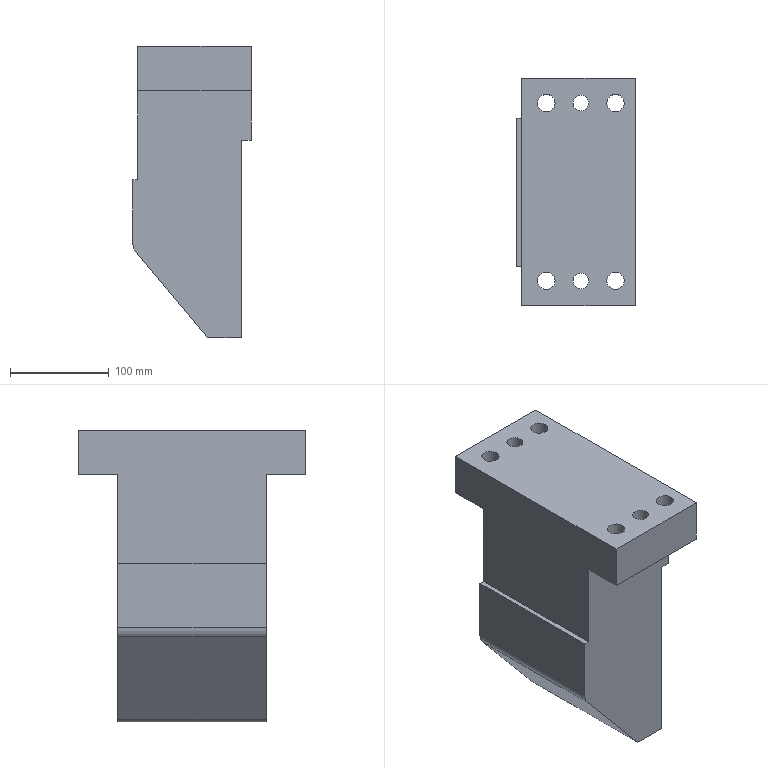Part | NX | features solid 2 | 1 solid | 31 faces | box 120 x 230 x 295 mm | volume 4727759 mm3 | plane 19 | cylinder 12 | commonest cylinder face diameters 17.5 x4 26 x4 16 x2 10 x1 30 x1
STEP:
#1=CARTESIAN_POINT('',(785.,300.,35.));
#2=VERTEX_POINT('',#1);
#3=CARTESIAN_POINT('',(785.,70.,35.));
#4=VERTEX_POINT('',#3);
#5=CARTESIAN_POINT('',(785.,82.5,35.));
#6=DIRECTION('',(0.,1.,0.));
#7=VECTOR('',#6,1000.);
#8=LINE('',#5,#7);
#9=EDGE_CURVE('',#2,#4,#8,.F.);
#10=ORIENTED_EDGE('',*,*,#9,.F.);
#11=CARTESIAN_POINT('',(785.,300.,-10.));
#12=VERTEX_POINT('',#11);
#13=CARTESIAN_POINT('',(785.,300.,-158.));
#14=DIRECTION('',(0.,0.,-1.));
#15=VECTOR('',#14,1000.);
#16=LINE('',#13,#15);
#17=EDGE_CURVE('',#2,#12,#16,.T.);
#18=ORIENTED_EDGE('',*,*,#17,.T.);
#19=CARTESIAN_POINT('',(785.,260.,-10.));
#20=VERTEX_POINT('',#19);
#21=CARTESIAN_POINT('',(785.,383.5,-10.));
#22=DIRECTION('',(0.,1.,0.));
#23=VECTOR('',#22,1000.);
#24=LINE('',#21,#23);
#25=EDGE_CURVE('',#12,#20,#24,.F.);
#26=ORIENTED_EDGE('',*,*,#25,.T.);
#27=CARTESIAN_POINT('',(785.,260.,-100.));
#28=VERTEX_POINT('',#27);
#29=CARTESIAN_POINT('',(785.,260.,-334.604));
#30=DIRECTION('',(0.,0.,-1.));
#31=VECTOR('',#30,1000.);
#32=LINE('',#29,#31);
#33=EDGE_CURVE('',#20,#28,#32,.T.);
#34=ORIENTED_EDGE('',*,*,#33,.T.);
#35=CARTESIAN_POINT('',(785.,110.,-100.));
#36=VERTEX_POINT('',#35);
#37=CARTESIAN_POINT('',(785.,340.,-100.));
#38=DIRECTION('',(0.,-1.,0.));
#39=VECTOR('',#38,1000.);
#40=LINE('',#37,#39);
#41=EDGE_CURVE('',#28,#36,#40,.T.);
#42=ORIENTED_EDGE('',*,*,#41,.T.);
#43=CARTESIAN_POINT('',(785.,110.,-10.));
#44=VERTEX_POINT('',#43);
#45=CARTESIAN_POINT('',(785.,110.,-334.604));
#46=DIRECTION('',(0.,0.,-1.));
#47=VECTOR('',#46,1000.);
#48=LINE('',#45,#47);
#49=EDGE_CURVE('',#44,#36,#48,.T.);
#50=ORIENTED_EDGE('',*,*,#49,.F.);
#51=CARTESIAN_POINT('',(785.,70.,-10.));
#52=VERTEX_POINT('',#51);
#53=CARTESIAN_POINT('',(785.,21.5,-10.));
#54=DIRECTION('',(0.,-1.,0.));
#55=VECTOR('',#54,1000.);
#56=LINE('',#53,#55);
#57=EDGE_CURVE('',#52,#44,#56,.F.);
#58=ORIENTED_EDGE('',*,*,#57,.F.);
#59=CARTESIAN_POINT('',(785.,70.,-158.));
#60=DIRECTION('',(0.,0.,-1.));
#61=VECTOR('',#60,1000.);
#62=LINE('',#59,#61);
#63=EDGE_CURVE('',#4,#52,#62,.T.);
#64=ORIENTED_EDGE('',*,*,#63,.F.);
#65=EDGE_LOOP('',(#10,#18,#26,#34,#42,#50,#58,#64));
#66=FACE_BOUND('',#65,.T.);
#67=CARTESIAN_POINT('',(785.,82.5,-158.));
#68=DIRECTION('',(-1.,0.,0.));
#69=DIRECTION('',(0.,0.,-1.));
#70=AXIS2_PLACEMENT_3D('',#67,#68,#69);
#71=PLANE('',#70);
#72=ADVANCED_FACE('',(#66),#71,.T.);
#73=CARTESIAN_POINT('',(900.,70.,35.));
#74=VERTEX_POINT('',#73);
#75=CARTESIAN_POINT('',(900.,300.,35.));
#76=VERTEX_POINT('',#75);
#77=CARTESIAN_POINT('',(900.,82.5,35.));
#78=DIRECTION('',(0.,-1.,0.));
#79=VECTOR('',#78,1000.);
#80=LINE('',#77,#79);
#81=EDGE_CURVE('',#74,#76,#80,.F.);
#82=ORIENTED_EDGE('',*,*,#81,.T.);
#83=CARTESIAN_POINT('',(785.,300.,35.));
#84=DIRECTION('',(-1.,0.,0.));
#85=VECTOR('',#84,1000.);
#86=LINE('',#83,#85);
#87=EDGE_CURVE('',#2,#76,#86,.F.);
#88=ORIENTED_EDGE('',*,*,#87,.F.);
#89=ORIENTED_EDGE('',*,*,#9,.T.);
#90=CARTESIAN_POINT('',(785.,70.,35.));
#91=DIRECTION('',(-1.,0.,0.));
#92=VECTOR('',#91,1000.);
#93=LINE('',#90,#92);
#94=EDGE_CURVE('',#4,#74,#93,.F.);
#95=ORIENTED_EDGE('',*,*,#94,.T.);
#96=EDGE_LOOP('',(#82,#88,#89,#95));
#97=FACE_BOUND('',#96,.T.);
#98=CARTESIAN_POINT('',(801.25,275.,35.));
#99=VERTEX_POINT('',#98);
#100=CARTESIAN_POINT('',(810.,275.,35.));
#101=DIRECTION('',(0.,0.,1.));
#102=DIRECTION('',(-1.,0.,0.));
#103=AXIS2_PLACEMENT_3D('',#100,#101,#102);
#104=CIRCLE('',#103,8.75);
#105=EDGE_CURVE('',#99,#99,#104,.F.);
#106=ORIENTED_EDGE('',*,*,#105,.T.);
#107=EDGE_LOOP('',(#106));
#108=FACE_BOUND('',#107,.T.);
#109=CARTESIAN_POINT('',(871.25,275.,35.));
#110=VERTEX_POINT('',#109);
#111=CARTESIAN_POINT('',(880.,275.,35.));
#112=DIRECTION('',(0.,0.,1.));
#113=DIRECTION('',(-1.,0.,0.));
#114=AXIS2_PLACEMENT_3D('',#111,#112,#113);
#115=CIRCLE('',#114,8.75);
#116=EDGE_CURVE('',#110,#110,#115,.F.);
#117=ORIENTED_EDGE('',*,*,#116,.T.);
#118=EDGE_LOOP('',(#117));
#119=FACE_BOUND('',#118,.T.);
#120=CARTESIAN_POINT('',(837.,275.,35.));
#121=VERTEX_POINT('',#120);
#122=CARTESIAN_POINT('',(845.,275.,35.));
#123=DIRECTION('',(0.,0.,1.));
#124=DIRECTION('',(-1.,0.,0.));
#125=AXIS2_PLACEMENT_3D('',#122,#123,#124);
#126=CIRCLE('',#125,8.);
#127=EDGE_CURVE('',#121,#121,#126,.F.);
#128=ORIENTED_EDGE('',*,*,#127,.T.);
#129=EDGE_LOOP('',(#128));
#130=FACE_BOUND('',#129,.T.);
#131=CARTESIAN_POINT('',(837.,95.,35.));
#132=VERTEX_POINT('',#131);
#133=CARTESIAN_POINT('',(845.,95.,35.));
#134=DIRECTION('',(0.,0.,-1.));
#135=DIRECTION('',(-1.,0.,0.));
#136=AXIS2_PLACEMENT_3D('',#133,#134,#135);
#137=CIRCLE('',#136,8.);
#138=EDGE_CURVE('',#132,#132,#137,.F.);
#139=ORIENTED_EDGE('',*,*,#138,.F.);
#140=EDGE_LOOP('',(#139));
#141=FACE_BOUND('',#140,.T.);
#142=CARTESIAN_POINT('',(871.25,95.,35.));
#143=VERTEX_POINT('',#142);
#144=CARTESIAN_POINT('',(880.,95.,35.));
#145=DIRECTION('',(0.,0.,-1.));
#146=DIRECTION('',(-1.,0.,0.));
#147=AXIS2_PLACEMENT_3D('',#144,#145,#146);
#148=CIRCLE('',#147,8.75);
#149=EDGE_CURVE('',#143,#143,#148,.F.);
#150=ORIENTED_EDGE('',*,*,#149,.F.);
#151=EDGE_LOOP('',(#150));
#152=FACE_BOUND('',#151,.T.);
#153=CARTESIAN_POINT('',(801.25,95.,35.));
#154=VERTEX_POINT('',#153);
#155=CARTESIAN_POINT('',(810.,95.,35.));
#156=DIRECTION('',(0.,0.,-1.));
#157=DIRECTION('',(-1.,0.,0.));
#158=AXIS2_PLACEMENT_3D('',#155,#156,#157);
#159=CIRCLE('',#158,8.75);
#160=EDGE_CURVE('',#154,#154,#159,.F.);
#161=ORIENTED_EDGE('',*,*,#160,.F.);
#162=EDGE_LOOP('',(#161));
#163=FACE_BOUND('',#162,.T.);
#164=CARTESIAN_POINT('',(800.,82.5,35.));
#165=DIRECTION('',(0.,0.,1.));
#166=DIRECTION('',(-1.,0.,0.));
#167=AXIS2_PLACEMENT_3D('',#164,#165,#166);
#168=PLANE('',#167);
#169=ADVANCED_FACE('',(#97,#108,#119,#130,#141,#152,#163),#168,.T.);
#170=CARTESIAN_POINT('',(900.,260.,-60.));
#171=VERTEX_POINT('',#170);
#172=CARTESIAN_POINT('',(900.,260.,-10.));
#173=VERTEX_POINT('',#172);
#174=CARTESIAN_POINT('',(900.,260.,37.));
#175=DIRECTION('',(0.,0.,1.));
#176=VECTOR('',#175,1000.);
#177=LINE('',#174,#176);
#178=EDGE_CURVE('',#171,#173,#177,.T.);
#179=ORIENTED_EDGE('',*,*,#178,.T.);
#180=CARTESIAN_POINT('',(900.,300.,-10.));
#181=VERTEX_POINT('',#180);
#182=CARTESIAN_POINT('',(900.,383.5,-10.));
#183=DIRECTION('',(0.,-1.,0.));
#184=VECTOR('',#183,1000.);
#185=LINE('',#182,#184);
#186=EDGE_CURVE('',#181,#173,#185,.T.);
#187=ORIENTED_EDGE('',*,*,#186,.F.);
#188=CARTESIAN_POINT('',(900.,300.,37.));
#189=DIRECTION('',(0.,0.,-1.));
#190=VECTOR('',#189,1000.);
#191=LINE('',#188,#190);
#192=EDGE_CURVE('',#76,#181,#191,.T.);
#193=ORIENTED_EDGE('',*,*,#192,.F.);
#194=ORIENTED_EDGE('',*,*,#81,.F.);
#195=CARTESIAN_POINT('',(900.,70.,-10.));
#196=VERTEX_POINT('',#195);
#197=CARTESIAN_POINT('',(900.,70.,37.));
#198=DIRECTION('',(0.,0.,-1.));
#199=VECTOR('',#198,1000.);
#200=LINE('',#197,#199);
#201=EDGE_CURVE('',#74,#196,#200,.T.);
#202=ORIENTED_EDGE('',*,*,#201,.T.);
#203=CARTESIAN_POINT('',(900.,110.,-10.));
#204=VERTEX_POINT('',#203);
#205=CARTESIAN_POINT('',(900.,172.5,-10.));
#206=DIRECTION('',(0.,1.,0.));
#207=VECTOR('',#206,1000.);
#208=LINE('',#205,#207);
#209=EDGE_CURVE('',#196,#204,#208,.T.);
#210=ORIENTED_EDGE('',*,*,#209,.T.);
#211=CARTESIAN_POINT('',(900.,110.,-60.));
#212=VERTEX_POINT('',#211);
#213=CARTESIAN_POINT('',(900.,110.,-334.604));
#214=DIRECTION('',(0.,0.,-1.));
#215=VECTOR('',#214,1000.);
#216=LINE('',#213,#215);
#217=EDGE_CURVE('',#204,#212,#216,.T.);
#218=ORIENTED_EDGE('',*,*,#217,.T.);
#219=CARTESIAN_POINT('',(900.,282.5,-60.));
#220=DIRECTION('',(0.,1.,0.));
#221=VECTOR('',#220,1000.);
#222=LINE('',#219,#221);
#223=EDGE_CURVE('',#212,#171,#222,.T.);
#224=ORIENTED_EDGE('',*,*,#223,.T.);
#225=EDGE_LOOP('',(#179,#187,#193,#194,#202,#210,#218,#224));
#226=FACE_BOUND('',#225,.T.);
#227=CARTESIAN_POINT('',(900.,172.5,37.));
#228=DIRECTION('',(-1.,0.,0.));
#229=DIRECTION('',(0.,0.,-1.));
#230=AXIS2_PLACEMENT_3D('',#227,#228,#229);
#231=PLANE('',#230);
#232=ADVANCED_FACE('',(#226),#231,.F.);
#233=CARTESIAN_POINT('',(695.,110.,-10.));
#234=DIRECTION('',(1.,0.,0.));
#235=VECTOR('',#234,1000.);
#236=LINE('',#233,#235);
#237=EDGE_CURVE('',#44,#204,#236,.T.);
#238=ORIENTED_EDGE('',*,*,#237,.F.);
#239=ORIENTED_EDGE('',*,*,#49,.T.);
#240=CARTESIAN_POINT('',(780.,110.,-100.));
#241=VERTEX_POINT('',#240);
#242=CARTESIAN_POINT('',(840.,110.,-100.));
#243=DIRECTION('',(1.,0.,0.));
#244=VECTOR('',#243,1000.);
#245=LINE('',#242,#244);
#246=EDGE_CURVE('',#241,#36,#245,.T.);
#247=ORIENTED_EDGE('',*,*,#246,.F.);
#248=CARTESIAN_POINT('',(780.,110.,-164.54));
#249=VERTEX_POINT('',#248);
#250=CARTESIAN_POINT('',(780.,110.,-334.604));
#251=DIRECTION('',(0.,0.,-1.));
#252=VECTOR('',#251,1000.);
#253=LINE('',#250,#252);
#254=EDGE_CURVE('',#241,#249,#253,.T.);
#255=ORIENTED_EDGE('',*,*,#254,.T.);
#256=CARTESIAN_POINT('',(783.509,110.,-174.182));
#257=VERTEX_POINT('',#256);
#258=CARTESIAN_POINT('',(795.,110.,-164.54));
#259=DIRECTION('',(0.,-1.,0.));
#260=DIRECTION('',(0.,0.,1.));
#261=AXIS2_PLACEMENT_3D('',#258,#259,#260);
#262=CIRCLE('',#261,15.);
#263=EDGE_CURVE('',#249,#257,#262,.T.);
#264=ORIENTED_EDGE('',*,*,#263,.T.);
#265=CARTESIAN_POINT('',(854.02,110.,-258.214));
#266=VERTEX_POINT('',#265);
#267=CARTESIAN_POINT('',(780.,110.,-170.));
#268=DIRECTION('',(0.6428,0.,-0.766));
#269=VECTOR('',#268,1000.);
#270=LINE('',#267,#269);
#271=EDGE_CURVE('',#257,#266,#270,.T.);
#272=ORIENTED_EDGE('',*,*,#271,.T.);
#273=CARTESIAN_POINT('',(857.851,110.,-260.));
#274=VERTEX_POINT('',#273);
#275=CARTESIAN_POINT('',(857.851,110.,-255.));
#276=DIRECTION('',(0.,-1.,0.));
#277=DIRECTION('',(0.,0.,1.));
#278=AXIS2_PLACEMENT_3D('',#275,#276,#277);
#279=CIRCLE('',#278,5.);
#280=EDGE_CURVE('',#266,#274,#279,.T.);
#281=ORIENTED_EDGE('',*,*,#280,.T.);
#282=CARTESIAN_POINT('',(890.,110.,-260.));
#283=VERTEX_POINT('',#282);
#284=CARTESIAN_POINT('',(764.279,110.,-260.));
#285=DIRECTION('',(1.,0.,0.));
#286=VECTOR('',#285,1000.);
#287=LINE('',#284,#286);
#288=EDGE_CURVE('',#274,#283,#287,.T.);
#289=ORIENTED_EDGE('',*,*,#288,.T.);
#290=CARTESIAN_POINT('',(890.,110.,-60.));
#291=VERTEX_POINT('',#290);
#292=CARTESIAN_POINT('',(890.,110.,-334.604));
#293=DIRECTION('',(0.,0.,1.));
#294=VECTOR('',#293,1000.);
#295=LINE('',#292,#294);
#296=EDGE_CURVE('',#283,#291,#295,.T.);
#297=ORIENTED_EDGE('',*,*,#296,.T.);
#298=CARTESIAN_POINT('',(764.279,110.,-60.));
#299=DIRECTION('',(1.,0.,0.));
#300=VECTOR('',#299,1000.);
#301=LINE('',#298,#300);
#302=EDGE_CURVE('',#291,#212,#301,.T.);
#303=ORIENTED_EDGE('',*,*,#302,.T.);
#304=ORIENTED_EDGE('',*,*,#217,.F.);
#305=EDGE_LOOP('',(#238,#239,#247,#255,#264,#272,#281,#289,#297,#303,#304));
#306=FACE_BOUND('',#305,.T.);
#307=CARTESIAN_POINT('',(764.279,110.,-334.604));
#308=DIRECTION('',(0.,-1.,0.));
#309=DIRECTION('',(0.,0.,1.));
#310=AXIS2_PLACEMENT_3D('',#307,#308,#309);
#311=PLANE('',#310);
#312=ADVANCED_FACE('',(#306),#311,.T.);
#313=ORIENTED_EDGE('',*,*,#33,.F.);
#314=CARTESIAN_POINT('',(695.,260.,-10.));
#315=DIRECTION('',(1.,0.,0.));
#316=VECTOR('',#315,1000.);
#317=LINE('',#314,#316);
#318=EDGE_CURVE('',#20,#173,#317,.T.);
#319=ORIENTED_EDGE('',*,*,#318,.T.);
#320=ORIENTED_EDGE('',*,*,#178,.F.);
#321=CARTESIAN_POINT('',(890.,260.,-60.));
#322=VERTEX_POINT('',#321);
#323=CARTESIAN_POINT('',(935.,260.,-60.));
#324=DIRECTION('',(-1.,0.,0.));
#325=VECTOR('',#324,1000.);
#326=LINE('',#323,#325);
#327=EDGE_CURVE('',#171,#322,#326,.T.);
#328=ORIENTED_EDGE('',*,*,#327,.T.);
#329=CARTESIAN_POINT('',(890.,260.,-260.));
#330=VERTEX_POINT('',#329);
#331=CARTESIAN_POINT('',(890.,260.,-334.604));
#332=DIRECTION('',(0.,0.,1.));
#333=VECTOR('',#332,1000.);
#334=LINE('',#331,#333);
#335=EDGE_CURVE('',#330,#322,#334,.T.);
#336=ORIENTED_EDGE('',*,*,#335,.F.);
#337=CARTESIAN_POINT('',(857.851,260.,-260.));
#338=VERTEX_POINT('',#337);
#339=CARTESIAN_POINT('',(764.279,260.,-260.));
#340=DIRECTION('',(1.,0.,0.));
#341=VECTOR('',#340,1000.);
#342=LINE('',#339,#341);
#343=EDGE_CURVE('',#338,#330,#342,.T.);
#344=ORIENTED_EDGE('',*,*,#343,.F.);
#345=CARTESIAN_POINT('',(854.02,260.,-258.214));
#346=VERTEX_POINT('',#345);
#347=CARTESIAN_POINT('',(857.851,260.,-255.));
#348=DIRECTION('',(0.,-1.,0.));
#349=DIRECTION('',(0.,0.,1.));
#350=AXIS2_PLACEMENT_3D('',#347,#348,#349);
#351=CIRCLE('',#350,5.);
#352=EDGE_CURVE('',#338,#346,#351,.F.);
#353=ORIENTED_EDGE('',*,*,#352,.T.);
#354=CARTESIAN_POINT('',(783.509,260.,-174.182));
#355=VERTEX_POINT('',#354);
#356=CARTESIAN_POINT('',(780.,260.,-170.));
#357=DIRECTION('',(0.6428,0.,-0.766));
#358=VECTOR('',#357,1000.);
#359=LINE('',#356,#358);
#360=EDGE_CURVE('',#355,#346,#359,.T.);
#361=ORIENTED_EDGE('',*,*,#360,.F.);
#362=CARTESIAN_POINT('',(780.,260.,-164.54));
#363=VERTEX_POINT('',#362);
#364=CARTESIAN_POINT('',(795.,260.,-164.54));
#365=DIRECTION('',(0.,-1.,0.));
#366=DIRECTION('',(0.,0.,1.));
#367=AXIS2_PLACEMENT_3D('',#364,#365,#366);
#368=CIRCLE('',#367,15.);
#369=EDGE_CURVE('',#355,#363,#368,.F.);
#370=ORIENTED_EDGE('',*,*,#369,.T.);
#371=CARTESIAN_POINT('',(780.,260.,-100.));
#372=VERTEX_POINT('',#371);
#373=CARTESIAN_POINT('',(780.,260.,-334.604));
#374=DIRECTION('',(0.,0.,-1.));
#375=VECTOR('',#374,1000.);
#376=LINE('',#373,#375);
#377=EDGE_CURVE('',#372,#363,#376,.T.);
#378=ORIENTED_EDGE('',*,*,#377,.F.);
#379=CARTESIAN_POINT('',(764.279,260.,-100.));
#380=DIRECTION('',(-1.,0.,0.));
#381=VECTOR('',#380,1000.);
#382=LINE('',#379,#381);
#383=EDGE_CURVE('',#28,#372,#382,.T.);
#384=ORIENTED_EDGE('',*,*,#383,.F.);
#385=EDGE_LOOP('',(#313,#319,#320,#328,#336,#344,#353,#361,#370,#378,#384));
#386=FACE_BOUND('',#385,.T.);
#387=CARTESIAN_POINT('',(764.279,260.,-334.604));
#388=DIRECTION('',(0.,-1.,0.));
#389=DIRECTION('',(0.,0.,1.));
#390=AXIS2_PLACEMENT_3D('',#387,#388,#389);
#391=PLANE('',#390);
#392=ADVANCED_FACE('',(#386),#391,.F.);
#393=ORIENTED_EDGE('',*,*,#288,.F.);
#394=CARTESIAN_POINT('',(857.851,315.,-260.));
#395=DIRECTION('',(0.,1.,0.));
#396=VECTOR('',#395,1000.);
#397=LINE('',#394,#396);
#398=EDGE_CURVE('',#274,#338,#397,.T.);
#399=ORIENTED_EDGE('',*,*,#398,.T.);
#400=ORIENTED_EDGE('',*,*,#343,.T.);
#401=CARTESIAN_POINT('',(890.,172.5,-260.));
#402=DIRECTION('',(0.,1.,0.));
#403=VECTOR('',#402,1000.);
#404=LINE('',#401,#403);
#405=EDGE_CURVE('',#283,#330,#404,.T.);
#406=ORIENTED_EDGE('',*,*,#405,.F.);
#407=EDGE_LOOP('',(#393,#399,#400,#406));
#408=FACE_BOUND('',#407,.T.);
#409=CARTESIAN_POINT('',(1145.969,-8.5,-260.));
#410=DIRECTION('',(0.,0.,-1.));
#411=DIRECTION('',(0.,-1.,0.));
#412=AXIS2_PLACEMENT_3D('',#409,#410,#411);
#413=PLANE('',#412);
#414=ADVANCED_FACE('',(#408),#413,.T.);
#415=ORIENTED_EDGE('',*,*,#335,.T.);
#416=CARTESIAN_POINT('',(890.,172.5,-60.));
#417=DIRECTION('',(0.,1.,0.));
#418=VECTOR('',#417,1000.);
#419=LINE('',#416,#418);
#420=EDGE_CURVE('',#291,#322,#419,.T.);
#421=ORIENTED_EDGE('',*,*,#420,.F.);
#422=ORIENTED_EDGE('',*,*,#296,.F.);
#423=ORIENTED_EDGE('',*,*,#405,.T.);
#424=EDGE_LOOP('',(#415,#421,#422,#423));
#425=FACE_BOUND('',#424,.T.);
#426=CARTESIAN_POINT('',(890.,172.5,-453.));
#427=DIRECTION('',(1.,0.,0.));
#428=DIRECTION('',(0.,0.,1.));
#429=AXIS2_PLACEMENT_3D('',#426,#427,#428);
#430=PLANE('',#429);
#431=ADVANCED_FACE('',(#425),#430,.T.);
#432=ORIENTED_EDGE('',*,*,#327,.F.);
#433=ORIENTED_EDGE('',*,*,#223,.F.);
#434=ORIENTED_EDGE('',*,*,#302,.F.);
#435=ORIENTED_EDGE('',*,*,#420,.T.);
#436=EDGE_LOOP('',(#432,#433,#434,#435));
#437=FACE_BOUND('',#436,.T.);
#438=CARTESIAN_POINT('',(935.,282.5,-60.));
#439=DIRECTION('',(0.,0.,-1.));
#440=DIRECTION('',(0.,1.,0.));
#441=AXIS2_PLACEMENT_3D('',#438,#439,#440);
#442=PLANE('',#441);
#443=ADVANCED_FACE('',(#437),#442,.T.);
#444=ORIENTED_EDGE('',*,*,#377,.T.);
#445=CARTESIAN_POINT('',(780.,135.,-164.54));
#446=DIRECTION('',(0.,-1.,0.));
#447=VECTOR('',#446,1000.);
#448=LINE('',#445,#447);
#449=EDGE_CURVE('',#363,#249,#448,.T.);
#450=ORIENTED_EDGE('',*,*,#449,.T.);
#451=ORIENTED_EDGE('',*,*,#254,.F.);
#452=CARTESIAN_POINT('',(780.,340.,-100.));
#453=DIRECTION('',(0.,1.,0.));
#454=VECTOR('',#453,1000.);
#455=LINE('',#452,#454);
#456=EDGE_CURVE('',#372,#241,#455,.F.);
#457=ORIENTED_EDGE('',*,*,#456,.F.);
#458=EDGE_LOOP('',(#444,#450,#451,#457));
#459=FACE_BOUND('',#458,.T.);
#460=CARTESIAN_POINT('',(780.,340.,-95.));
#461=DIRECTION('',(-1.,0.,0.));
#462=DIRECTION('',(0.,1.,0.));
#463=AXIS2_PLACEMENT_3D('',#460,#461,#462);
#464=PLANE('',#463);
#465=ADVANCED_FACE('',(#459),#464,.T.);
#466=ORIENTED_EDGE('',*,*,#271,.F.);
#467=CARTESIAN_POINT('',(783.509,265.,-174.182));
#468=DIRECTION('',(0.,-1.,0.));
#469=VECTOR('',#468,1000.);
#470=LINE('',#467,#469);
#471=EDGE_CURVE('',#257,#355,#470,.F.);
#472=ORIENTED_EDGE('',*,*,#471,.T.);
#473=ORIENTED_EDGE('',*,*,#360,.T.);
#474=CARTESIAN_POINT('',(854.02,165.,-258.214));
#475=DIRECTION('',(0.,1.,0.));
#476=VECTOR('',#475,1000.);
#477=LINE('',#474,#476);
#478=EDGE_CURVE('',#346,#266,#477,.F.);
#479=ORIENTED_EDGE('',*,*,#478,.T.);
#480=EDGE_LOOP('',(#466,#472,#473,#479));
#481=FACE_BOUND('',#480,.T.);
#482=CARTESIAN_POINT('',(780.,215.,-170.));
#483=DIRECTION('',(0.766,0.,0.6428));
#484=DIRECTION('',(-0.6428,0.,0.766));
#485=AXIS2_PLACEMENT_3D('',#482,#483,#484);
#486=PLANE('',#485);
#487=ADVANCED_FACE('',(#481),#486,.F.);
#488=ORIENTED_EDGE('',*,*,#246,.T.);
#489=ORIENTED_EDGE('',*,*,#41,.F.);
#490=ORIENTED_EDGE('',*,*,#383,.T.);
#491=ORIENTED_EDGE('',*,*,#456,.T.);
#492=EDGE_LOOP('',(#488,#489,#490,#491));
#493=FACE_BOUND('',#492,.T.);
#494=CARTESIAN_POINT('',(840.,340.,-100.));
#495=DIRECTION('',(0.,0.,1.));
#496=DIRECTION('',(0.,1.,0.));
#497=AXIS2_PLACEMENT_3D('',#494,#495,#496);
#498=PLANE('',#497);
#499=ADVANCED_FACE('',(#493),#498,.T.);
#500=ORIENTED_EDGE('',*,*,#280,.F.);
#501=ORIENTED_EDGE('',*,*,#478,.F.);
#502=ORIENTED_EDGE('',*,*,#352,.F.);
#503=ORIENTED_EDGE('',*,*,#398,.F.);
#504=EDGE_LOOP('',(#500,#501,#502,#503));
#505=FACE_BOUND('',#504,.T.);
#506=CARTESIAN_POINT('',(857.851,245.,-255.));
#507=DIRECTION('',(0.,-1.,0.));
#508=DIRECTION('',(0.,0.,-1.));
#509=AXIS2_PLACEMENT_3D('',#506,#507,#508);
#510=CYLINDRICAL_SURFACE('',#509,5.);
#511=ADVANCED_FACE('',(#505),#510,.T.);
#512=ORIENTED_EDGE('',*,*,#369,.F.);
#513=ORIENTED_EDGE('',*,*,#471,.F.);
#514=ORIENTED_EDGE('',*,*,#263,.F.);
#515=ORIENTED_EDGE('',*,*,#449,.F.);
#516=EDGE_LOOP('',(#512,#513,#514,#515));
#517=FACE_BOUND('',#516,.T.);
#518=CARTESIAN_POINT('',(795.,340.,-164.54));
#519=DIRECTION('',(0.,1.,0.));
#520=DIRECTION('',(0.,0.,-1.));
#521=AXIS2_PLACEMENT_3D('',#518,#519,#520);
#522=CYLINDRICAL_SURFACE('',#521,15.);
#523=ADVANCED_FACE('',(#517),#522,.T.);
#524=CARTESIAN_POINT('',(801.25,275.,10.));
#525=VERTEX_POINT('',#524);
#526=CARTESIAN_POINT('',(810.,275.,10.));
#527=DIRECTION('',(0.,0.,1.));
#528=DIRECTION('',(-1.,0.,0.));
#529=AXIS2_PLACEMENT_3D('',#526,#527,#528);
#530=CIRCLE('',#529,8.75);
#531=EDGE_CURVE('',#525,#525,#530,.T.);
#532=ORIENTED_EDGE('',*,*,#531,.T.);
#533=EDGE_LOOP('',(#532));
#534=FACE_BOUND('',#533,.T.);
#535=CARTESIAN_POINT('',(797.,275.,10.));
#536=VERTEX_POINT('',#535);
#537=CARTESIAN_POINT('',(810.,275.,10.));
#538=DIRECTION('',(0.,0.,1.));
#539=DIRECTION('',(-1.,0.,0.));
#540=AXIS2_PLACEMENT_3D('',#537,#538,#539);
#541=CIRCLE('',#540,13.);
#542=EDGE_CURVE('',#536,#536,#541,.T.);
#543=ORIENTED_EDGE('',*,*,#542,.F.);
#544=EDGE_LOOP('',(#543));
#545=FACE_BOUND('',#544,.T.);
#546=CARTESIAN_POINT('',(725.,323.5,10.));
#547=DIRECTION('',(0.,0.,1.));
#548=DIRECTION('',(-1.,0.,0.));
#549=AXIS2_PLACEMENT_3D('',#546,#547,#548);
#550=PLANE('',#549);
#551=ADVANCED_FACE('',(#534,#545),#550,.F.);
#552=CARTESIAN_POINT('',(871.25,275.,10.));
#553=VERTEX_POINT('',#552);
#554=CARTESIAN_POINT('',(880.,275.,10.));
#555=DIRECTION('',(0.,0.,1.));
#556=DIRECTION('',(-1.,0.,0.));
#557=AXIS2_PLACEMENT_3D('',#554,#555,#556);
#558=CIRCLE('',#557,8.75);
#559=EDGE_CURVE('',#553,#553,#558,.T.);
#560=ORIENTED_EDGE('',*,*,#559,.T.);
#561=EDGE_LOOP('',(#560));
#562=FACE_BOUND('',#561,.T.);
#563=CARTESIAN_POINT('',(867.,275.,10.));
#564=VERTEX_POINT('',#563);
#565=CARTESIAN_POINT('',(880.,275.,10.));
#566=DIRECTION('',(0.,0.,1.));
#567=DIRECTION('',(-1.,0.,0.));
#568=AXIS2_PLACEMENT_3D('',#565,#566,#567);
#569=CIRCLE('',#568,13.);
#570=EDGE_CURVE('',#564,#564,#569,.T.);
#571=ORIENTED_EDGE('',*,*,#570,.F.);
#572=EDGE_LOOP('',(#571));
#573=FACE_BOUND('',#572,.T.);
#574=CARTESIAN_POINT('',(840.,323.5,10.));
#575=DIRECTION('',(0.,0.,1.));
#576=DIRECTION('',(-1.,0.,0.));
#577=AXIS2_PLACEMENT_3D('',#574,#575,#576);
#578=PLANE('',#577);
#579=ADVANCED_FACE('',(#562,#573),#578,.F.);
#580=ORIENTED_EDGE('',*,*,#559,.F.);
#581=EDGE_LOOP('',(#580));
#582=FACE_BOUND('',#581,.T.);
#583=ORIENTED_EDGE('',*,*,#116,.F.);
#584=EDGE_LOOP('',(#583));
#585=FACE_BOUND('',#584,.T.);
#586=CARTESIAN_POINT('',(880.,275.,87.));
#587=DIRECTION('',(0.,0.,1.));
#588=DIRECTION('',(-1.,0.,0.));
#589=AXIS2_PLACEMENT_3D('',#586,#587,#588);
#590=CYLINDRICAL_SURFACE('',#589,8.75);
#591=ADVANCED_FACE('',(#582,#585),#590,.F.);
#592=ORIENTED_EDGE('',*,*,#531,.F.);
#593=EDGE_LOOP('',(#592));
#594=FACE_BOUND('',#593,.T.);
#595=ORIENTED_EDGE('',*,*,#105,.F.);
#596=EDGE_LOOP('',(#595));
#597=FACE_BOUND('',#596,.T.);
#598=CARTESIAN_POINT('',(810.,275.,87.));
#599=DIRECTION('',(0.,0.,1.));
#600=DIRECTION('',(-1.,0.,0.));
#601=AXIS2_PLACEMENT_3D('',#598,#599,#600);
#602=CYLINDRICAL_SURFACE('',#601,8.75);
#603=ADVANCED_FACE('',(#594,#597),#602,.F.);
#604=CARTESIAN_POINT('',(797.,275.,-10.));
#605=VERTEX_POINT('',#604);
#606=CARTESIAN_POINT('',(810.,275.,-10.));
#607=DIRECTION('',(0.,0.,1.));
#608=DIRECTION('',(-1.,0.,0.));
#609=AXIS2_PLACEMENT_3D('',#606,#607,#608);
#610=CIRCLE('',#609,13.);
#611=EDGE_CURVE('',#605,#605,#610,.F.);
#612=ORIENTED_EDGE('',*,*,#611,.T.);
#613=EDGE_LOOP('',(#612));
#614=FACE_BOUND('',#613,.T.);
#615=ORIENTED_EDGE('',*,*,#542,.T.);
#616=EDGE_LOOP('',(#615));
#617=FACE_BOUND('',#616,.T.);
#618=CARTESIAN_POINT('',(810.,275.,-13.));
#619=DIRECTION('',(0.,0.,1.));
#620=DIRECTION('',(-1.,0.,0.));
#621=AXIS2_PLACEMENT_3D('',#618,#619,#620);
#622=CYLINDRICAL_SURFACE('',#621,13.);
#623=ADVANCED_FACE('',(#614,#617),#622,.F.);
#624=CARTESIAN_POINT('',(837.,275.,-10.));
#625=VERTEX_POINT('',#624);
#626=CARTESIAN_POINT('',(845.,275.,-10.));
#627=DIRECTION('',(0.,0.,1.));
#628=DIRECTION('',(-1.,0.,0.));
#629=AXIS2_PLACEMENT_3D('',#626,#627,#628);
#630=CIRCLE('',#629,8.);
#631=EDGE_CURVE('',#625,#625,#630,.F.);
#632=ORIENTED_EDGE('',*,*,#631,.T.);
#633=EDGE_LOOP('',(#632));
#634=FACE_BOUND('',#633,.T.);
#635=ORIENTED_EDGE('',*,*,#127,.F.);
#636=EDGE_LOOP('',(#635));
#637=FACE_BOUND('',#636,.T.);
#638=CARTESIAN_POINT('',(845.,275.,-13.));
#639=DIRECTION('',(0.,0.,1.));
#640=DIRECTION('',(-1.,0.,0.));
#641=AXIS2_PLACEMENT_3D('',#638,#639,#640);
#642=CYLINDRICAL_SURFACE('',#641,8.);
#643=ADVANCED_FACE('',(#634,#637),#642,.F.);
#644=CARTESIAN_POINT('',(867.,275.,-10.));
#645=VERTEX_POINT('',#644);
#646=CARTESIAN_POINT('',(880.,275.,-10.));
#647=DIRECTION('',(0.,0.,1.));
#648=DIRECTION('',(-1.,0.,0.));
#649=AXIS2_PLACEMENT_3D('',#646,#647,#648);
#650=CIRCLE('',#649,13.);
#651=EDGE_CURVE('',#645,#645,#650,.F.);
#652=ORIENTED_EDGE('',*,*,#651,.T.);
#653=EDGE_LOOP('',(#652));
#654=FACE_BOUND('',#653,.T.);
#655=ORIENTED_EDGE('',*,*,#570,.T.);
#656=EDGE_LOOP('',(#655));
#657=FACE_BOUND('',#656,.T.);
#658=CARTESIAN_POINT('',(880.,275.,-13.));
#659=DIRECTION('',(0.,0.,1.));
#660=DIRECTION('',(-1.,0.,0.));
#661=AXIS2_PLACEMENT_3D('',#658,#659,#660);
#662=CYLINDRICAL_SURFACE('',#661,13.);
#663=ADVANCED_FACE('',(#654,#657),#662,.F.);
#664=CARTESIAN_POINT('',(749.279,300.,-10.));
#665=DIRECTION('',(1.,0.,0.));
#666=VECTOR('',#665,1000.);
#667=LINE('',#664,#666);
#668=EDGE_CURVE('',#12,#181,#667,.T.);
#669=ORIENTED_EDGE('',*,*,#668,.F.);
#670=ORIENTED_EDGE('',*,*,#17,.F.);
#671=ORIENTED_EDGE('',*,*,#87,.T.);
#672=ORIENTED_EDGE('',*,*,#192,.T.);
#673=EDGE_LOOP('',(#669,#670,#671,#672));
#674=FACE_BOUND('',#673,.T.);
#675=CARTESIAN_POINT('',(749.279,300.,37.));
#676=DIRECTION('',(0.,1.,0.));
#677=DIRECTION('',(0.,0.,-1.));
#678=AXIS2_PLACEMENT_3D('',#675,#676,#677);
#679=PLANE('',#678);
#680=ADVANCED_FACE('',(#674),#679,.T.);
#681=ORIENTED_EDGE('',*,*,#668,.T.);
#682=ORIENTED_EDGE('',*,*,#186,.T.);
#683=ORIENTED_EDGE('',*,*,#318,.F.);
#684=ORIENTED_EDGE('',*,*,#25,.F.);
#685=EDGE_LOOP('',(#681,#682,#683,#684));
#686=FACE_BOUND('',#685,.T.);
#687=ORIENTED_EDGE('',*,*,#651,.F.);
#688=EDGE_LOOP('',(#687));
#689=FACE_BOUND('',#688,.T.);
#690=ORIENTED_EDGE('',*,*,#631,.F.);
#691=EDGE_LOOP('',(#690));
#692=FACE_BOUND('',#691,.T.);
#693=ORIENTED_EDGE('',*,*,#611,.F.);
#694=EDGE_LOOP('',(#693));
#695=FACE_BOUND('',#694,.T.);
#696=CARTESIAN_POINT('',(695.,383.5,-10.));
#697=DIRECTION('',(0.,0.,1.));
#698=DIRECTION('',(-1.,0.,0.));
#699=AXIS2_PLACEMENT_3D('',#696,#697,#698);
#700=PLANE('',#699);
#701=ADVANCED_FACE('',(#686,#689,#692,#695),#700,.F.);
#702=CARTESIAN_POINT('',(801.25,95.,10.));
#703=VERTEX_POINT('',#702);
#704=CARTESIAN_POINT('',(810.,95.,10.));
#705=DIRECTION('',(0.,0.,-1.));
#706=DIRECTION('',(-1.,0.,0.));
#707=AXIS2_PLACEMENT_3D('',#704,#705,#706);
#708=CIRCLE('',#707,8.75);
#709=EDGE_CURVE('',#703,#703,#708,.T.);
#710=ORIENTED_EDGE('',*,*,#709,.F.);
#711=EDGE_LOOP('',(#710));
#712=FACE_BOUND('',#711,.T.);
#713=CARTESIAN_POINT('',(797.,95.,10.));
#714=VERTEX_POINT('',#713);
#715=CARTESIAN_POINT('',(810.,95.,10.));
#716=DIRECTION('',(0.,0.,-1.));
#717=DIRECTION('',(-1.,0.,0.));
#718=AXIS2_PLACEMENT_3D('',#715,#716,#717);
#719=CIRCLE('',#718,13.);
#720=EDGE_CURVE('',#714,#714,#719,.T.);
#721=ORIENTED_EDGE('',*,*,#720,.T.);
#722=EDGE_LOOP('',(#721));
#723=FACE_BOUND('',#722,.T.);
#724=CARTESIAN_POINT('',(725.,81.5,10.));
#725=DIRECTION('',(0.,0.,1.));
#726=DIRECTION('',(-1.,0.,0.));
#727=AXIS2_PLACEMENT_3D('',#724,#725,#726);
#728=PLANE('',#727);
#729=ADVANCED_FACE('',(#712,#723),#728,.F.);
#730=CARTESIAN_POINT('',(871.25,95.,10.));
#731=VERTEX_POINT('',#730);
#732=CARTESIAN_POINT('',(880.,95.,10.));
#733=DIRECTION('',(0.,0.,-1.));
#734=DIRECTION('',(-1.,0.,0.));
#735=AXIS2_PLACEMENT_3D('',#732,#733,#734);
#736=CIRCLE('',#735,8.75);
#737=EDGE_CURVE('',#731,#731,#736,.T.);
#738=ORIENTED_EDGE('',*,*,#737,.F.);
#739=EDGE_LOOP('',(#738));
#740=FACE_BOUND('',#739,.T.);
#741=CARTESIAN_POINT('',(867.,95.,10.));
#742=VERTEX_POINT('',#741);
#743=CARTESIAN_POINT('',(880.,95.,10.));
#744=DIRECTION('',(0.,0.,-1.));
#745=DIRECTION('',(-1.,0.,0.));
#746=AXIS2_PLACEMENT_3D('',#743,#744,#745);
#747=CIRCLE('',#746,13.);
#748=EDGE_CURVE('',#742,#742,#747,.T.);
#749=ORIENTED_EDGE('',*,*,#748,.T.);
#750=EDGE_LOOP('',(#749));
#751=FACE_BOUND('',#750,.T.);
#752=CARTESIAN_POINT('',(840.,81.5,10.));
#753=DIRECTION('',(0.,0.,1.));
#754=DIRECTION('',(-1.,0.,0.));
#755=AXIS2_PLACEMENT_3D('',#752,#753,#754);
#756=PLANE('',#755);
#757=ADVANCED_FACE('',(#740,#751),#756,.F.);
#758=ORIENTED_EDGE('',*,*,#709,.T.);
#759=EDGE_LOOP('',(#758));
#760=FACE_BOUND('',#759,.T.);
#761=ORIENTED_EDGE('',*,*,#160,.T.);
#762=EDGE_LOOP('',(#761));
#763=FACE_BOUND('',#762,.T.);
#764=CARTESIAN_POINT('',(810.,95.,87.));
#765=DIRECTION('',(0.,0.,1.));
#766=DIRECTION('',(-1.,0.,0.));
#767=AXIS2_PLACEMENT_3D('',#764,#765,#766);
#768=CYLINDRICAL_SURFACE('',#767,8.75);
#769=ADVANCED_FACE('',(#760,#763),#768,.F.);
#770=ORIENTED_EDGE('',*,*,#737,.T.);
#771=EDGE_LOOP('',(#770));
#772=FACE_BOUND('',#771,.T.);
#773=ORIENTED_EDGE('',*,*,#149,.T.);
#774=EDGE_LOOP('',(#773));
#775=FACE_BOUND('',#774,.T.);
#776=CARTESIAN_POINT('',(880.,95.,87.));
#777=DIRECTION('',(0.,0.,1.));
#778=DIRECTION('',(-1.,0.,0.));
#779=AXIS2_PLACEMENT_3D('',#776,#777,#778);
#780=CYLINDRICAL_SURFACE('',#779,8.75);
#781=ADVANCED_FACE('',(#772,#775),#780,.F.);
#782=CARTESIAN_POINT('',(797.,95.,-10.));
#783=VERTEX_POINT('',#782);
#784=CARTESIAN_POINT('',(810.,95.,-10.));
#785=DIRECTION('',(0.,0.,-1.));
#786=DIRECTION('',(-1.,0.,0.));
#787=AXIS2_PLACEMENT_3D('',#784,#785,#786);
#788=CIRCLE('',#787,13.);
#789=EDGE_CURVE('',#783,#783,#788,.F.);
#790=ORIENTED_EDGE('',*,*,#789,.F.);
#791=EDGE_LOOP('',(#790));
#792=FACE_BOUND('',#791,.T.);
#793=ORIENTED_EDGE('',*,*,#720,.F.);
#794=EDGE_LOOP('',(#793));
#795=FACE_BOUND('',#794,.T.);
#796=CARTESIAN_POINT('',(810.,95.,-13.));
#797=DIRECTION('',(0.,0.,1.));
#798=DIRECTION('',(-1.,0.,0.));
#799=AXIS2_PLACEMENT_3D('',#796,#797,#798);
#800=CYLINDRICAL_SURFACE('',#799,13.);
#801=ADVANCED_FACE('',(#792,#795),#800,.F.);
#802=CARTESIAN_POINT('',(837.,95.,-10.));
#803=VERTEX_POINT('',#802);
#804=CARTESIAN_POINT('',(845.,95.,-10.));
#805=DIRECTION('',(0.,0.,-1.));
#806=DIRECTION('',(-1.,0.,0.));
#807=AXIS2_PLACEMENT_3D('',#804,#805,#806);
#808=CIRCLE('',#807,8.);
#809=EDGE_CURVE('',#803,#803,#808,.F.);
#810=ORIENTED_EDGE('',*,*,#809,.F.);
#811=EDGE_LOOP('',(#810));
#812=FACE_BOUND('',#811,.T.);
#813=ORIENTED_EDGE('',*,*,#138,.T.);
#814=EDGE_LOOP('',(#813));
#815=FACE_BOUND('',#814,.T.);
#816=CARTESIAN_POINT('',(845.,95.,-13.));
#817=DIRECTION('',(0.,0.,1.));
#818=DIRECTION('',(-1.,0.,0.));
#819=AXIS2_PLACEMENT_3D('',#816,#817,#818);
#820=CYLINDRICAL_SURFACE('',#819,8.);
#821=ADVANCED_FACE('',(#812,#815),#820,.F.);
#822=CARTESIAN_POINT('',(867.,95.,-10.));
#823=VERTEX_POINT('',#822);
#824=CARTESIAN_POINT('',(880.,95.,-10.));
#825=DIRECTION('',(0.,0.,-1.));
#826=DIRECTION('',(-1.,0.,0.));
#827=AXIS2_PLACEMENT_3D('',#824,#825,#826);
#828=CIRCLE('',#827,13.);
#829=EDGE_CURVE('',#823,#823,#828,.F.);
#830=ORIENTED_EDGE('',*,*,#829,.F.);
#831=EDGE_LOOP('',(#830));
#832=FACE_BOUND('',#831,.T.);
#833=ORIENTED_EDGE('',*,*,#748,.F.);
#834=EDGE_LOOP('',(#833));
#835=FACE_BOUND('',#834,.T.);
#836=CARTESIAN_POINT('',(880.,95.,-13.));
#837=DIRECTION('',(0.,0.,1.));
#838=DIRECTION('',(-1.,0.,0.));
#839=AXIS2_PLACEMENT_3D('',#836,#837,#838);
#840=CYLINDRICAL_SURFACE('',#839,13.);
#841=ADVANCED_FACE('',(#832,#835),#840,.F.);
#842=CARTESIAN_POINT('',(749.279,70.,-10.));
#843=DIRECTION('',(1.,0.,0.));
#844=VECTOR('',#843,1000.);
#845=LINE('',#842,#844);
#846=EDGE_CURVE('',#52,#196,#845,.T.);
#847=ORIENTED_EDGE('',*,*,#846,.T.);
#848=ORIENTED_EDGE('',*,*,#201,.F.);
#849=ORIENTED_EDGE('',*,*,#94,.F.);
#850=ORIENTED_EDGE('',*,*,#63,.T.);
#851=EDGE_LOOP('',(#847,#848,#849,#850));
#852=FACE_BOUND('',#851,.T.);
#853=CARTESIAN_POINT('',(749.279,70.,37.));
#854=DIRECTION('',(0.,-1.,0.));
#855=DIRECTION('',(0.,0.,-1.));
#856=AXIS2_PLACEMENT_3D('',#853,#854,#855);
#857=PLANE('',#856);
#858=ADVANCED_FACE('',(#852),#857,.T.);
#859=ORIENTED_EDGE('',*,*,#846,.F.);
#860=ORIENTED_EDGE('',*,*,#57,.T.);
#861=ORIENTED_EDGE('',*,*,#237,.T.);
#862=ORIENTED_EDGE('',*,*,#209,.F.);
#863=EDGE_LOOP('',(#859,#860,#861,#862));
#864=FACE_BOUND('',#863,.T.);
#865=ORIENTED_EDGE('',*,*,#829,.T.);
#866=EDGE_LOOP('',(#865));
#867=FACE_BOUND('',#866,.T.);
#868=ORIENTED_EDGE('',*,*,#809,.T.);
#869=EDGE_LOOP('',(#868));
#870=FACE_BOUND('',#869,.T.);
#871=ORIENTED_EDGE('',*,*,#789,.T.);
#872=EDGE_LOOP('',(#871));
#873=FACE_BOUND('',#872,.T.);
#874=CARTESIAN_POINT('',(695.,21.5,-10.));
#875=DIRECTION('',(0.,0.,1.));
#876=DIRECTION('',(-1.,0.,0.));
#877=AXIS2_PLACEMENT_3D('',#874,#875,#876);
#878=PLANE('',#877);
#879=ADVANCED_FACE('',(#864,#867,#870,#873),#878,.F.);
#880=CLOSED_SHELL('',(#72,#169,#232,#312,#392,#414,#431,#443,#465,#487,#499,#511,#523,#551,#579,#591,#603,#623,#643,#663,#680,#701,#729,#757,#769,#781,#801,#821,#841,#858,#879));
#881=MANIFOLD_SOLID_BREP('',#880);
#882=(LENGTH_UNIT()NAMED_UNIT(*)SI_UNIT(.MILLI.,.METRE.));
#883=UNCERTAINTY_MEASURE_WITH_UNIT(LENGTH_MEASURE(0.00001),#882,'','');
#884=(NAMED_UNIT(*)PLANE_ANGLE_UNIT()SI_UNIT($,.RADIAN.));
#885=(NAMED_UNIT(*)SI_UNIT($,.STERADIAN.)SOLID_ANGLE_UNIT());
#886=(GEOMETRIC_REPRESENTATION_CONTEXT(3)GLOBAL_UNCERTAINTY_ASSIGNED_CONTEXT((#883))GLOBAL_UNIT_ASSIGNED_CONTEXT((#882,#884,#885))REPRESENTATION_CONTEXT('',''));
#887=ADVANCED_BREP_SHAPE_REPRESENTATION('',(#881),#886);